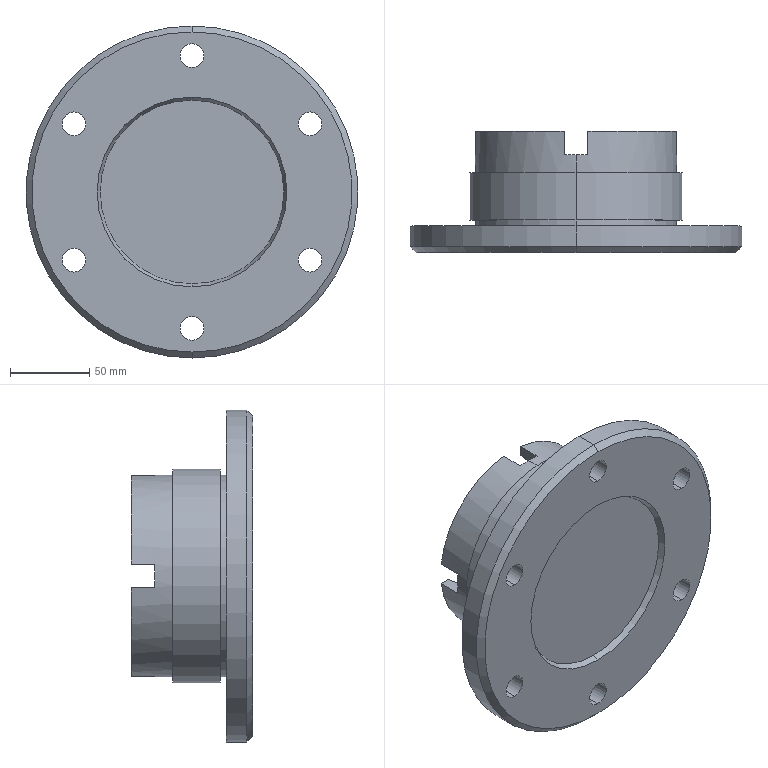Part | SolidWorks | features ICE 2, Revolution 1, Scale 1 | 1 solid | 50 faces | box 210 x 76.875 x 210 mm | volume 837773 mm3 | plane 22 | cylinder 20 | cone 6 | torus 2 | commonest cylinder face diameters 15 x12 127.5 x4 135 x2 210 x2